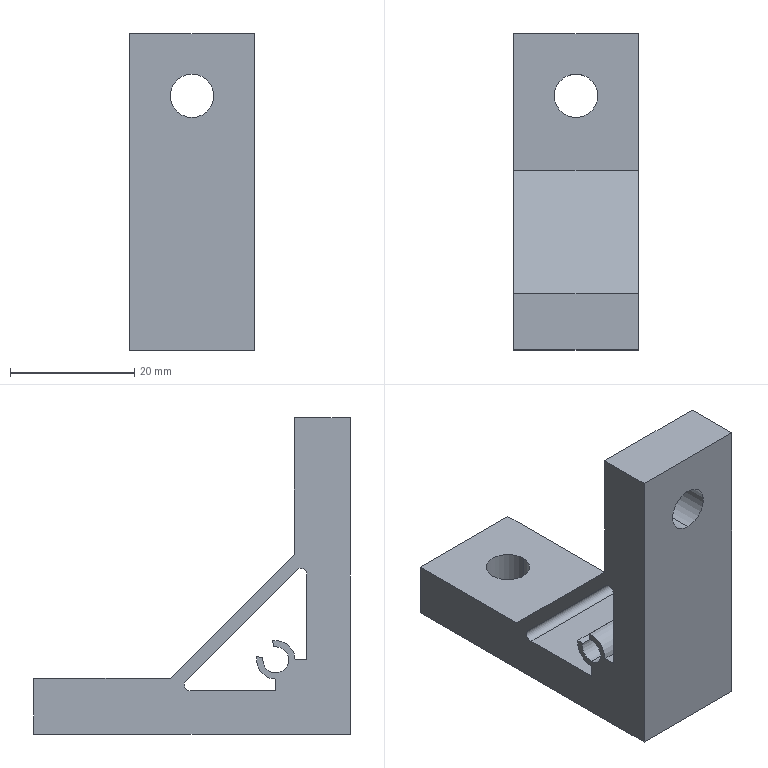Part | STEP file | hblts6_2_03 | 1 solid | 27 faces | box 20 x 51 x 51 mm | volume 16227 mm3 | plane 16 | cylinder 11 | commonest cylinder face diameters 7 x4 4.2 x3 2 x2 6.2 x2